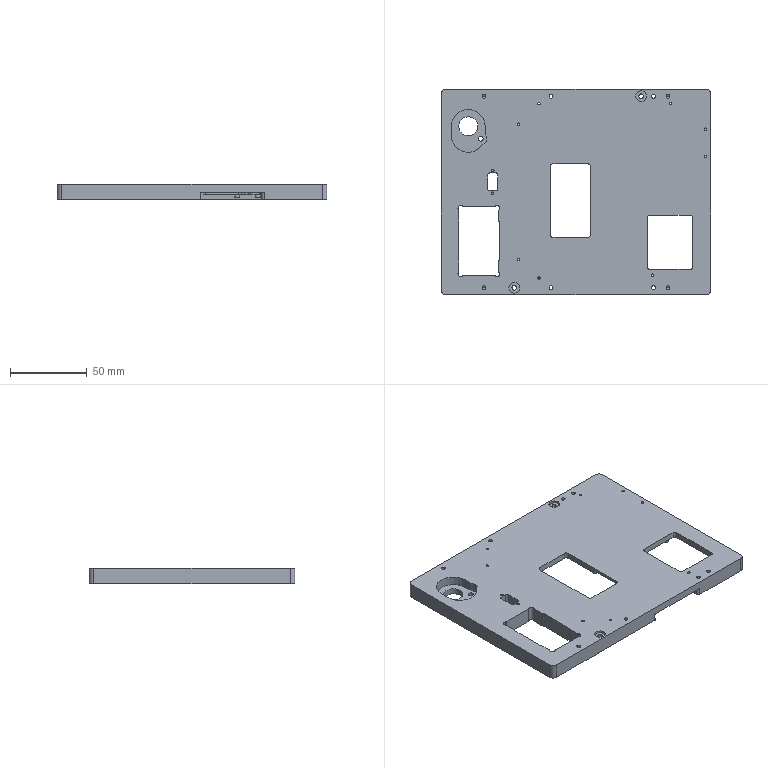Part | 1 solid | 387 faces | box 176 x 134 x 10 mm | volume 126907 mm3 | cylinder 222 | plane 136 | cone 29 | commonest cylinder face diameters 3.5 x65 3 x48 2.5 x21 1.6 x20 2 x16 8 x9